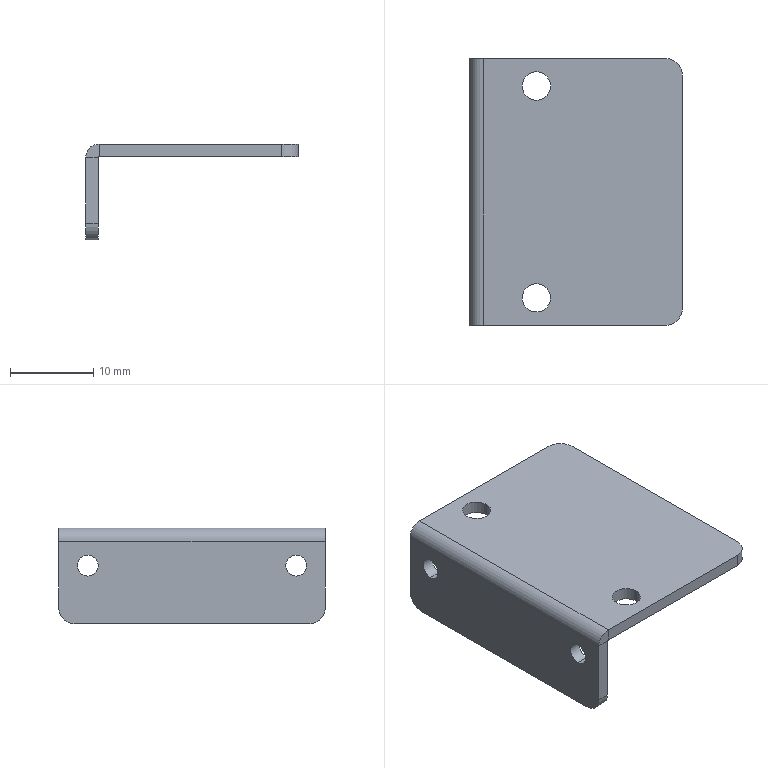Part | STEP file | lift photoelectric fixing plate | 1 solid | 26 faces | box 25.5 x 32 x 11.5 mm | volume 1639 mm3 | cylinder 14 | plane 12 | commonest cylinder face diameters 2.5 x4 3.4 x4 4 x4 0.2 x1 3.2 x1